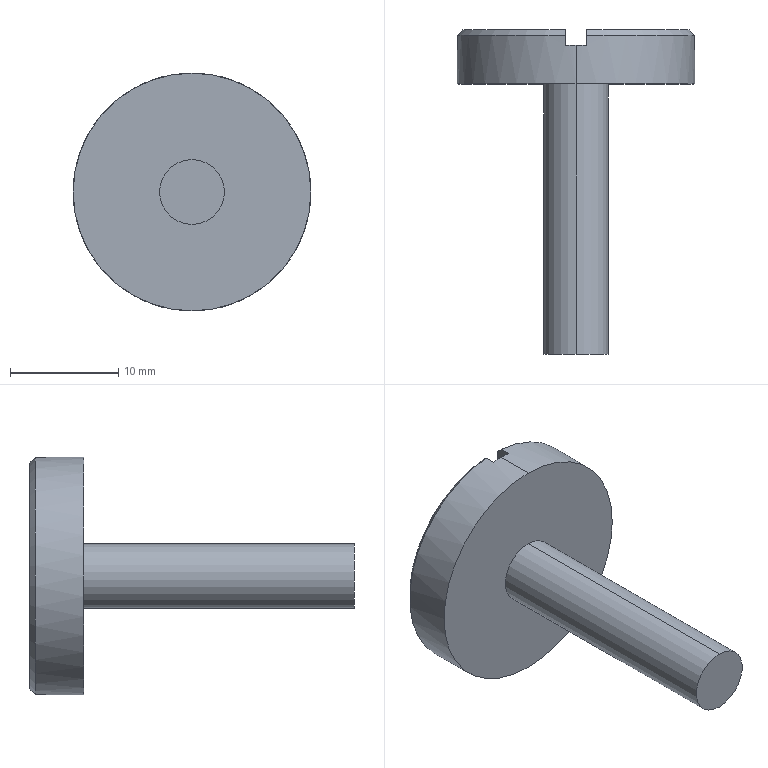Part | SolidWorks | features Chamfer 1, ICE 1, Revolution 1 | 1 solid | 13 faces | box 22 x 30 x 22 mm | volume 2536 mm3 | plane 7 | cylinder 4 | cone 2 | commonest cylinder face diameters 6 x2 22 x2
STEP:
#1=CARTESIAN_POINT('',(0.,-8.798,3.));
#2=VERTEX_POINT('',#1);
#3=CARTESIAN_POINT('',(0.,-8.798,-3.));
#4=VERTEX_POINT('',#3);
#5=CARTESIAN_POINT('',(0.,-8.798,0.));
#6=DIRECTION('',(0.,1.,0.));
#7=DIRECTION('',(0.,0.,1.));
#8=AXIS2_PLACEMENT_3D('',#5,#6,#7);
#9=CIRCLE('',#8,3.);
#10=EDGE_CURVE('',#2,#4,#9,.T.);
#11=ORIENTED_EDGE('',*,*,#10,.T.);
#12=CARTESIAN_POINT('',(0.,16.202,-3.));
#13=VERTEX_POINT('',#12);
#14=CARTESIAN_POINT('',(0.,28.351,-3.));
#15=DIRECTION('',(0.,1.,0.));
#16=VECTOR('',#15,1000.);
#17=LINE('',#14,#16);
#18=EDGE_CURVE('',#4,#13,#17,.T.);
#19=ORIENTED_EDGE('',*,*,#18,.T.);
#20=CARTESIAN_POINT('',(0.,16.202,3.));
#21=VERTEX_POINT('',#20);
#22=CARTESIAN_POINT('',(0.,16.202,0.));
#23=DIRECTION('',(0.,1.,0.));
#24=DIRECTION('',(0.,0.,1.));
#25=AXIS2_PLACEMENT_3D('',#22,#23,#24);
#26=CIRCLE('',#25,3.);
#27=EDGE_CURVE('',#21,#13,#26,.T.);
#28=ORIENTED_EDGE('',*,*,#27,.F.);
#29=CARTESIAN_POINT('',(0.,28.351,3.));
#30=DIRECTION('',(0.,1.,0.));
#31=VECTOR('',#30,1000.);
#32=LINE('',#29,#31);
#33=EDGE_CURVE('',#2,#21,#32,.T.);
#34=ORIENTED_EDGE('',*,*,#33,.F.);
#35=EDGE_LOOP('',(#11,#19,#28,#34));
#36=FACE_OUTER_BOUND('',#35,.T.);
#37=CARTESIAN_POINT('',(0.,28.351,0.));
#38=DIRECTION('',(0.,1.,0.));
#39=DIRECTION('',(0.,0.,1.));
#40=AXIS2_PLACEMENT_3D('',#37,#38,#39);
#41=CYLINDRICAL_SURFACE('',#40,3.);
#42=ADVANCED_FACE('',(#36),#41,.T.);
#43=CARTESIAN_POINT('',(0.,16.202,11.));
#44=VERTEX_POINT('',#43);
#45=CARTESIAN_POINT('',(0.,16.202,-11.));
#46=VERTEX_POINT('',#45);
#47=CARTESIAN_POINT('',(0.,16.202,0.));
#48=DIRECTION('',(0.,1.,0.));
#49=DIRECTION('',(0.,0.,1.));
#50=AXIS2_PLACEMENT_3D('',#47,#48,#49);
#51=CIRCLE('',#50,11.);
#52=EDGE_CURVE('',#44,#46,#51,.T.);
#53=ORIENTED_EDGE('',*,*,#52,.T.);
#54=CARTESIAN_POINT('',(0.,19.752,-11.));
#55=VERTEX_POINT('',#54);
#56=CARTESIAN_POINT('',(0.,28.351,-11.));
#57=DIRECTION('',(0.,1.,0.));
#58=VECTOR('',#57,1000.);
#59=LINE('',#56,#58);
#60=EDGE_CURVE('',#46,#55,#59,.T.);
#61=ORIENTED_EDGE('',*,*,#60,.T.);
#62=CARTESIAN_POINT('',(0.99,19.752,-10.955));
#63=VERTEX_POINT('',#62);
#64=CARTESIAN_POINT('',(0.,19.752,0.));
#65=DIRECTION('',(0.,1.,0.));
#66=DIRECTION('',(0.,0.,-1.));
#67=AXIS2_PLACEMENT_3D('',#64,#65,#66);
#68=CIRCLE('',#67,11.);
#69=EDGE_CURVE('',#63,#55,#68,.T.);
#70=ORIENTED_EDGE('',*,*,#69,.F.);
#71=CARTESIAN_POINT('',(0.99,20.702,-10.955));
#72=VERTEX_POINT('',#71);
#73=CARTESIAN_POINT('',(0.99,28.351,-10.955));
#74=DIRECTION('',(0.,-1.,0.));
#75=VECTOR('',#74,1000.);
#76=LINE('',#73,#75);
#77=EDGE_CURVE('',#72,#63,#76,.T.);
#78=ORIENTED_EDGE('',*,*,#77,.F.);
#79=CARTESIAN_POINT('',(0.99,20.702,10.955));
#80=VERTEX_POINT('',#79);
#81=CARTESIAN_POINT('',(0.,20.702,0.));
#82=DIRECTION('',(0.,-1.,0.));
#83=DIRECTION('',(0.,0.,1.));
#84=AXIS2_PLACEMENT_3D('',#81,#82,#83);
#85=CIRCLE('',#84,11.);
#86=EDGE_CURVE('',#72,#80,#85,.T.);
#87=ORIENTED_EDGE('',*,*,#86,.T.);
#88=CARTESIAN_POINT('',(0.99,19.752,10.955));
#89=VERTEX_POINT('',#88);
#90=CARTESIAN_POINT('',(0.99,28.351,10.955));
#91=DIRECTION('',(0.,1.,0.));
#92=VECTOR('',#91,1000.);
#93=LINE('',#90,#92);
#94=EDGE_CURVE('',#89,#80,#93,.T.);
#95=ORIENTED_EDGE('',*,*,#94,.F.);
#96=CARTESIAN_POINT('',(0.,19.752,11.));
#97=VERTEX_POINT('',#96);
#98=CARTESIAN_POINT('',(0.,19.752,0.));
#99=DIRECTION('',(0.,1.,0.));
#100=DIRECTION('',(0.,0.,-1.));
#101=AXIS2_PLACEMENT_3D('',#98,#99,#100);
#102=CIRCLE('',#101,11.);
#103=EDGE_CURVE('',#97,#89,#102,.T.);
#104=ORIENTED_EDGE('',*,*,#103,.F.);
#105=CARTESIAN_POINT('',(0.,28.351,11.));
#106=DIRECTION('',(0.,1.,0.));
#107=VECTOR('',#106,1000.);
#108=LINE('',#105,#107);
#109=EDGE_CURVE('',#44,#97,#108,.T.);
#110=ORIENTED_EDGE('',*,*,#109,.F.);
#111=EDGE_LOOP('',(#53,#61,#70,#78,#87,#95,#104,#110));
#112=FACE_OUTER_BOUND('',#111,.T.);
#113=CARTESIAN_POINT('',(0.,28.351,0.));
#114=DIRECTION('',(0.,1.,0.));
#115=DIRECTION('',(0.,0.,1.));
#116=AXIS2_PLACEMENT_3D('',#113,#114,#115);
#117=CYLINDRICAL_SURFACE('',#116,11.);
#118=ADVANCED_FACE('',(#112),#117,.T.);
#119=CARTESIAN_POINT('',(0.99,21.202,10.453));
#120=VERTEX_POINT('',#119);
#121=CARTESIAN_POINT('',(0.99,21.202,-10.453));
#122=VERTEX_POINT('',#121);
#123=CARTESIAN_POINT('',(0.99,21.202,0.));
#124=DIRECTION('',(0.,0.,-1.));
#125=VECTOR('',#124,1000.);
#126=LINE('',#123,#125);
#127=EDGE_CURVE('',#120,#122,#126,.T.);
#128=ORIENTED_EDGE('',*,*,#127,.F.);
#129=CARTESIAN_POINT('',(0.,21.202,0.));
#130=DIRECTION('',(0.,1.,0.));
#131=DIRECTION('',(0.,0.,1.));
#132=AXIS2_PLACEMENT_3D('',#129,#130,#131);
#133=CIRCLE('',#132,10.5);
#134=EDGE_CURVE('',#120,#122,#133,.T.);
#135=ORIENTED_EDGE('',*,*,#134,.T.);
#136=EDGE_LOOP('',(#128,#135));
#137=FACE_OUTER_BOUND('',#136,.T.);
#138=CARTESIAN_POINT('',(0.,21.202,0.));
#139=DIRECTION('',(0.,1.,0.));
#140=DIRECTION('',(0.,0.,1.));
#141=AXIS2_PLACEMENT_3D('',#138,#139,#140);
#142=PLANE('',#141);
#143=ADVANCED_FACE('',(#137),#142,.T.);
#144=CARTESIAN_POINT('',(-0.99,21.202,-10.453));
#145=VERTEX_POINT('',#144);
#146=CARTESIAN_POINT('',(-0.99,21.202,10.453));
#147=VERTEX_POINT('',#146);
#148=CARTESIAN_POINT('',(-0.99,21.202,0.));
#149=DIRECTION('',(0.,0.,1.));
#150=VECTOR('',#149,1000.);
#151=LINE('',#148,#150);
#152=EDGE_CURVE('',#145,#147,#151,.T.);
#153=ORIENTED_EDGE('',*,*,#152,.F.);
#154=CARTESIAN_POINT('',(0.,21.202,0.));
#155=DIRECTION('',(0.,1.,0.));
#156=DIRECTION('',(0.,0.,1.));
#157=AXIS2_PLACEMENT_3D('',#154,#155,#156);
#158=CIRCLE('',#157,10.5);
#159=EDGE_CURVE('',#145,#147,#158,.T.);
#160=ORIENTED_EDGE('',*,*,#159,.T.);
#161=EDGE_LOOP('',(#153,#160));
#162=FACE_OUTER_BOUND('',#161,.T.);
#163=CARTESIAN_POINT('',(0.,21.202,0.));
#164=DIRECTION('',(0.,1.,0.));
#165=DIRECTION('',(0.,0.,1.));
#166=AXIS2_PLACEMENT_3D('',#163,#164,#165);
#167=PLANE('',#166);
#168=ADVANCED_FACE('',(#162),#167,.T.);
#169=ORIENTED_EDGE('',*,*,#60,.F.);
#170=CARTESIAN_POINT('',(0.,16.202,0.));
#171=DIRECTION('',(0.,1.,0.));
#172=DIRECTION('',(0.,0.,1.));
#173=AXIS2_PLACEMENT_3D('',#170,#171,#172);
#174=CIRCLE('',#173,11.);
#175=EDGE_CURVE('',#46,#44,#174,.T.);
#176=ORIENTED_EDGE('',*,*,#175,.T.);
#177=ORIENTED_EDGE('',*,*,#109,.T.);
#178=CARTESIAN_POINT('',(-0.99,19.752,10.955));
#179=VERTEX_POINT('',#178);
#180=CARTESIAN_POINT('',(0.,19.752,0.));
#181=DIRECTION('',(0.,1.,0.));
#182=DIRECTION('',(0.,0.,-1.));
#183=AXIS2_PLACEMENT_3D('',#180,#181,#182);
#184=CIRCLE('',#183,11.);
#185=EDGE_CURVE('',#179,#97,#184,.T.);
#186=ORIENTED_EDGE('',*,*,#185,.F.);
#187=CARTESIAN_POINT('',(-0.99,20.702,10.955));
#188=VERTEX_POINT('',#187);
#189=CARTESIAN_POINT('',(-0.99,28.351,10.955));
#190=DIRECTION('',(0.,-1.,0.));
#191=VECTOR('',#190,1000.);
#192=LINE('',#189,#191);
#193=EDGE_CURVE('',#188,#179,#192,.T.);
#194=ORIENTED_EDGE('',*,*,#193,.F.);
#195=CARTESIAN_POINT('',(-0.99,20.702,-10.955));
#196=VERTEX_POINT('',#195);
#197=CARTESIAN_POINT('',(0.,20.702,0.));
#198=DIRECTION('',(0.,-1.,0.));
#199=DIRECTION('',(0.,0.,1.));
#200=AXIS2_PLACEMENT_3D('',#197,#198,#199);
#201=CIRCLE('',#200,11.);
#202=EDGE_CURVE('',#188,#196,#201,.T.);
#203=ORIENTED_EDGE('',*,*,#202,.T.);
#204=CARTESIAN_POINT('',(-0.99,19.752,-10.955));
#205=VERTEX_POINT('',#204);
#206=CARTESIAN_POINT('',(-0.99,28.351,-10.955));
#207=DIRECTION('',(0.,1.,0.));
#208=VECTOR('',#207,1000.);
#209=LINE('',#206,#208);
#210=EDGE_CURVE('',#205,#196,#209,.T.);
#211=ORIENTED_EDGE('',*,*,#210,.F.);
#212=CARTESIAN_POINT('',(0.,19.752,0.));
#213=DIRECTION('',(0.,1.,0.));
#214=DIRECTION('',(0.,0.,-1.));
#215=AXIS2_PLACEMENT_3D('',#212,#213,#214);
#216=CIRCLE('',#215,11.);
#217=EDGE_CURVE('',#55,#205,#216,.T.);
#218=ORIENTED_EDGE('',*,*,#217,.F.);
#219=EDGE_LOOP('',(#169,#176,#177,#186,#194,#203,#211,#218));
#220=FACE_OUTER_BOUND('',#219,.T.);
#221=CARTESIAN_POINT('',(0.,28.351,0.));
#222=DIRECTION('',(0.,1.,0.));
#223=DIRECTION('',(0.,0.,1.));
#224=AXIS2_PLACEMENT_3D('',#221,#222,#223);
#225=CYLINDRICAL_SURFACE('',#224,11.);
#226=ADVANCED_FACE('',(#220),#225,.T.);
#227=ORIENTED_EDGE('',*,*,#27,.T.);
#228=CARTESIAN_POINT('',(0.,16.202,0.));
#229=DIRECTION('',(0.,1.,0.));
#230=DIRECTION('',(0.,0.,1.));
#231=AXIS2_PLACEMENT_3D('',#228,#229,#230);
#232=CIRCLE('',#231,3.);
#233=EDGE_CURVE('',#13,#21,#232,.T.);
#234=ORIENTED_EDGE('',*,*,#233,.T.);
#235=EDGE_LOOP('',(#227,#234));
#236=FACE_BOUND('',#235,.T.);
#237=ORIENTED_EDGE('',*,*,#52,.F.);
#238=ORIENTED_EDGE('',*,*,#175,.F.);
#239=EDGE_LOOP('',(#237,#238));
#240=FACE_OUTER_BOUND('',#239,.T.);
#241=CARTESIAN_POINT('',(-11.,16.202,0.));
#242=DIRECTION('',(0.,-1.,0.));
#243=DIRECTION('',(0.,0.,-1.));
#244=AXIS2_PLACEMENT_3D('',#241,#242,#243);
#245=PLANE('',#244);
#246=ADVANCED_FACE('',(#236,#240),#245,.T.);
#247=ORIENTED_EDGE('',*,*,#18,.F.);
#248=CARTESIAN_POINT('',(0.,-8.798,0.));
#249=DIRECTION('',(0.,1.,0.));
#250=DIRECTION('',(0.,0.,1.));
#251=AXIS2_PLACEMENT_3D('',#248,#249,#250);
#252=CIRCLE('',#251,3.);
#253=EDGE_CURVE('',#4,#2,#252,.T.);
#254=ORIENTED_EDGE('',*,*,#253,.T.);
#255=ORIENTED_EDGE('',*,*,#33,.T.);
#256=ORIENTED_EDGE('',*,*,#233,.F.);
#257=EDGE_LOOP('',(#247,#254,#255,#256));
#258=FACE_OUTER_BOUND('',#257,.T.);
#259=CARTESIAN_POINT('',(0.,28.351,0.));
#260=DIRECTION('',(0.,1.,0.));
#261=DIRECTION('',(0.,0.,1.));
#262=AXIS2_PLACEMENT_3D('',#259,#260,#261);
#263=CYLINDRICAL_SURFACE('',#262,3.);
#264=ADVANCED_FACE('',(#258),#263,.T.);
#265=ORIENTED_EDGE('',*,*,#10,.F.);
#266=ORIENTED_EDGE('',*,*,#253,.F.);
#267=EDGE_LOOP('',(#265,#266));
#268=FACE_OUTER_BOUND('',#267,.T.);
#269=CARTESIAN_POINT('',(-3.,-8.798,0.));
#270=DIRECTION('',(0.,-1.,0.));
#271=DIRECTION('',(0.,0.,-1.));
#272=AXIS2_PLACEMENT_3D('',#269,#270,#271);
#273=PLANE('',#272);
#274=ADVANCED_FACE('',(#268),#273,.T.);
#275=ORIENTED_EDGE('',*,*,#127,.T.);
#276=CARTESIAN_POINT('',(0.99,21.202,-10.453));
#277=CARTESIAN_POINT('',(0.99,21.035,-10.621));
#278=CARTESIAN_POINT('',(0.99,20.869,-10.788));
#279=CARTESIAN_POINT('',(0.99,20.702,-10.955));
#280=B_SPLINE_CURVE_WITH_KNOTS('',3,(#276,#277,#278,#279),.UNSPECIFIED.,.F.,.F.,(4,4),(0.,0.0007086),.UNSPECIFIED.);
#281=EDGE_CURVE('',#122,#72,#280,.T.);
#282=ORIENTED_EDGE('',*,*,#281,.T.);
#283=ORIENTED_EDGE('',*,*,#77,.T.);
#284=CARTESIAN_POINT('',(0.99,19.752,-18.));
#285=DIRECTION('',(0.,0.,1.));
#286=VECTOR('',#285,1000.);
#287=LINE('',#284,#286);
#288=EDGE_CURVE('',#63,#89,#287,.T.);
#289=ORIENTED_EDGE('',*,*,#288,.T.);
#290=ORIENTED_EDGE('',*,*,#94,.T.);
#291=CARTESIAN_POINT('',(0.99,20.702,10.955));
#292=CARTESIAN_POINT('',(0.99,20.869,10.788));
#293=CARTESIAN_POINT('',(0.99,21.035,10.621));
#294=CARTESIAN_POINT('',(0.99,21.202,10.453));
#295=B_SPLINE_CURVE_WITH_KNOTS('',3,(#291,#292,#293,#294),.UNSPECIFIED.,.F.,.F.,(4,4),(0.,0.0007086),.UNSPECIFIED.);
#296=EDGE_CURVE('',#80,#120,#295,.T.);
#297=ORIENTED_EDGE('',*,*,#296,.T.);
#298=EDGE_LOOP('',(#275,#282,#283,#289,#290,#297));
#299=FACE_OUTER_BOUND('',#298,.T.);
#300=CARTESIAN_POINT('',(0.99,22.652,-18.));
#301=DIRECTION('',(1.,0.,0.));
#302=DIRECTION('',(0.,0.,-1.));
#303=AXIS2_PLACEMENT_3D('',#300,#301,#302);
#304=PLANE('',#303);
#305=ADVANCED_FACE('',(#299),#304,.F.);
#306=ORIENTED_EDGE('',*,*,#185,.T.);
#307=ORIENTED_EDGE('',*,*,#103,.T.);
#308=ORIENTED_EDGE('',*,*,#288,.F.);
#309=ORIENTED_EDGE('',*,*,#69,.T.);
#310=ORIENTED_EDGE('',*,*,#217,.T.);
#311=CARTESIAN_POINT('',(-0.99,19.752,-18.));
#312=DIRECTION('',(0.,0.,1.));
#313=VECTOR('',#312,1000.);
#314=LINE('',#311,#313);
#315=EDGE_CURVE('',#205,#179,#314,.T.);
#316=ORIENTED_EDGE('',*,*,#315,.T.);
#317=EDGE_LOOP('',(#306,#307,#308,#309,#310,#316));
#318=FACE_OUTER_BOUND('',#317,.T.);
#319=CARTESIAN_POINT('',(-0.99,19.752,-18.));
#320=DIRECTION('',(0.,-1.,0.));
#321=DIRECTION('',(0.,0.,-1.));
#322=AXIS2_PLACEMENT_3D('',#319,#320,#321);
#323=PLANE('',#322);
#324=ADVANCED_FACE('',(#318),#323,.F.);
#325=ORIENTED_EDGE('',*,*,#152,.T.);
#326=CARTESIAN_POINT('',(-0.99,21.202,10.453));
#327=CARTESIAN_POINT('',(-0.99,21.035,10.621));
#328=CARTESIAN_POINT('',(-0.99,20.869,10.788));
#329=CARTESIAN_POINT('',(-0.99,20.702,10.955));
#330=B_SPLINE_CURVE_WITH_KNOTS('',3,(#326,#327,#328,#329),.UNSPECIFIED.,.F.,.F.,(4,4),(0.,0.0007086),.UNSPECIFIED.);
#331=EDGE_CURVE('',#147,#188,#330,.T.);
#332=ORIENTED_EDGE('',*,*,#331,.T.);
#333=ORIENTED_EDGE('',*,*,#193,.T.);
#334=ORIENTED_EDGE('',*,*,#315,.F.);
#335=ORIENTED_EDGE('',*,*,#210,.T.);
#336=CARTESIAN_POINT('',(-0.99,20.702,-10.955));
#337=CARTESIAN_POINT('',(-0.99,20.869,-10.788));
#338=CARTESIAN_POINT('',(-0.99,21.035,-10.621));
#339=CARTESIAN_POINT('',(-0.99,21.202,-10.453));
#340=B_SPLINE_CURVE_WITH_KNOTS('',3,(#336,#337,#338,#339),.UNSPECIFIED.,.F.,.F.,(4,4),(0.,0.0007086),.UNSPECIFIED.);
#341=EDGE_CURVE('',#196,#145,#340,.T.);
#342=ORIENTED_EDGE('',*,*,#341,.T.);
#343=EDGE_LOOP('',(#325,#332,#333,#334,#335,#342));
#344=FACE_OUTER_BOUND('',#343,.T.);
#345=CARTESIAN_POINT('',(-0.99,22.652,-18.));
#346=DIRECTION('',(-1.,0.,0.));
#347=DIRECTION('',(0.,0.,1.));
#348=AXIS2_PLACEMENT_3D('',#345,#346,#347);
#349=PLANE('',#348);
#350=ADVANCED_FACE('',(#344),#349,.F.);
#351=ORIENTED_EDGE('',*,*,#296,.F.);
#352=ORIENTED_EDGE('',*,*,#86,.F.);
#353=ORIENTED_EDGE('',*,*,#281,.F.);
#354=ORIENTED_EDGE('',*,*,#134,.F.);
#355=EDGE_LOOP('',(#351,#352,#353,#354));
#356=FACE_OUTER_BOUND('',#355,.T.);
#357=CARTESIAN_POINT('',(0.,21.202,0.));
#358=DIRECTION('',(0.,-1.,0.));
#359=DIRECTION('',(0.,0.,-1.));
#360=AXIS2_PLACEMENT_3D('',#357,#358,#359);
#361=CONICAL_SURFACE('',#360,10.5,0.7854);
#362=ADVANCED_FACE('',(#356),#361,.T.);
#363=ORIENTED_EDGE('',*,*,#341,.F.);
#364=ORIENTED_EDGE('',*,*,#202,.F.);
#365=ORIENTED_EDGE('',*,*,#331,.F.);
#366=ORIENTED_EDGE('',*,*,#159,.F.);
#367=EDGE_LOOP('',(#363,#364,#365,#366));
#368=FACE_OUTER_BOUND('',#367,.T.);
#369=CARTESIAN_POINT('',(0.,21.202,0.));
#370=DIRECTION('',(0.,-1.,0.));
#371=DIRECTION('',(0.,0.,-1.));
#372=AXIS2_PLACEMENT_3D('',#369,#370,#371);
#373=CONICAL_SURFACE('',#372,10.5,0.7854);
#374=ADVANCED_FACE('',(#368),#373,.T.);
#375=CLOSED_SHELL('',(#42,#118,#143,#168,#226,#246,#264,#274,#305,#324,#350,#362,#374));
#376=MANIFOLD_SOLID_BREP('',#375);
#377=CARTESIAN_POINT('',(0.,0.,0.));
#378=DIRECTION('',(0.,0.,1.));
#379=DIRECTION('',(1.,0.,0.));
#380=AXIS2_PLACEMENT_3D('',#377,#378,#379);
#381=(LENGTH_UNIT()NAMED_UNIT(*)SI_UNIT(.MILLI.,.METRE.));
#382=UNCERTAINTY_MEASURE_WITH_UNIT(LENGTH_MEASURE(0.00001),#381,'','');
#383=(NAMED_UNIT(*)PLANE_ANGLE_UNIT()SI_UNIT($,.RADIAN.));
#384=(NAMED_UNIT(*)SI_UNIT($,.STERADIAN.)SOLID_ANGLE_UNIT());
#385=(GEOMETRIC_REPRESENTATION_CONTEXT(3)GLOBAL_UNCERTAINTY_ASSIGNED_CONTEXT((#382))GLOBAL_UNIT_ASSIGNED_CONTEXT((#381,#383,#384))REPRESENTATION_CONTEXT('',''));
#386=ADVANCED_BREP_SHAPE_REPRESENTATION('',(#376,#380),#385);